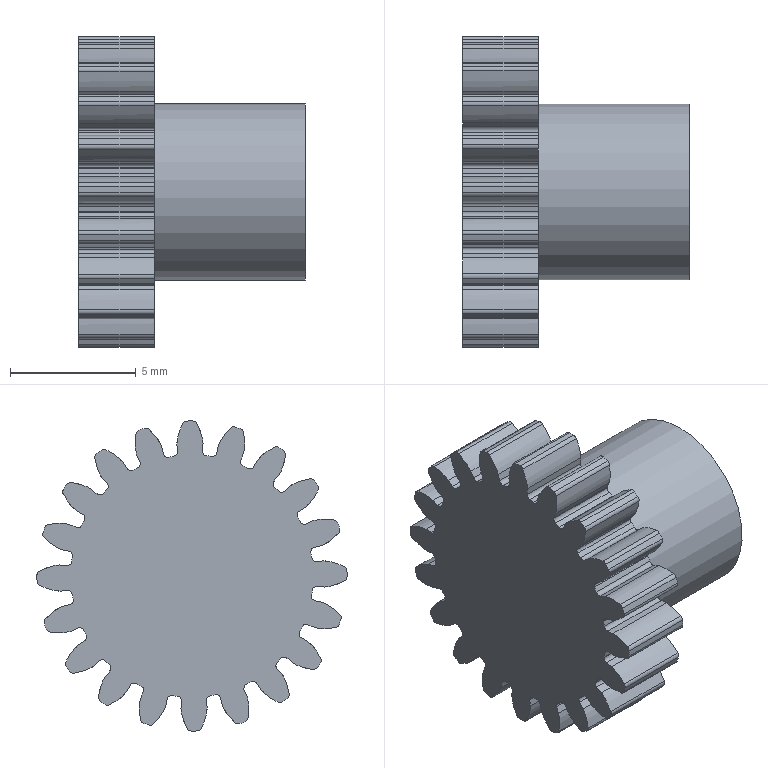Part | STEP file | Wytnij-wyci_gni_cie1_7 | 1 solid | 225 faces | box 9 x 12.32 x 12.32 mm | volume 463.728 mm3 | cylinder 139 | plane 46 | spline 40 | commonest cylinder face diameters 0.35 x96 9.632 x20 12.32 x20 4.86 x2 7 x1